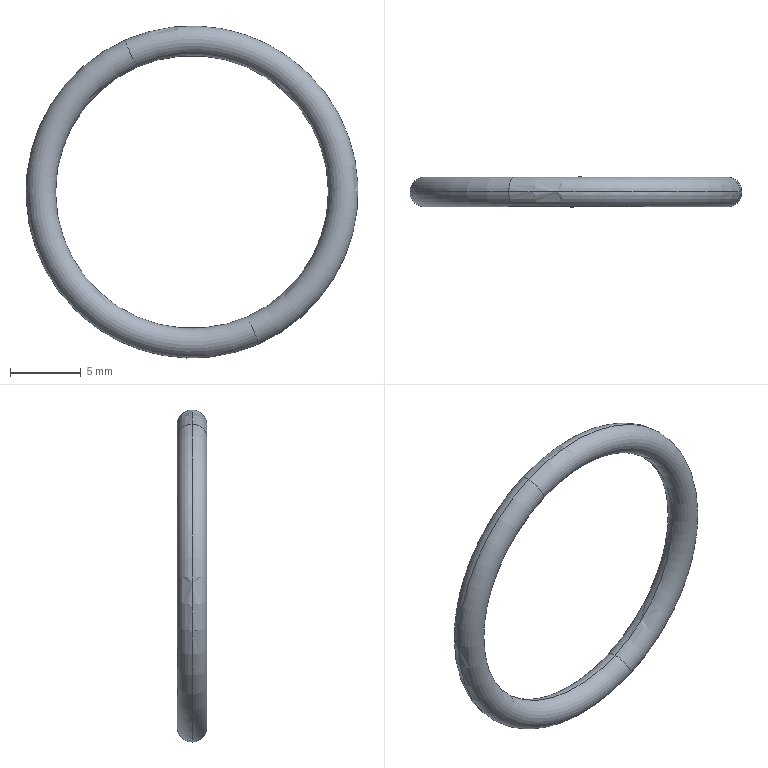Part | SolidWorks | features BaseBody 1 | 1 solid | 4 faces | box 23.5 x 2.1 x 23.5 mm | volume 232.859 mm3 | torus 4
STEP:
#1=CARTESIAN_POINT('',(224.737,118.05,10.742));
#2=VERTEX_POINT('',#1);
#3=CARTESIAN_POINT('',(225.589,118.05,8.822));
#4=VERTEX_POINT('',#3);
#5=CARTESIAN_POINT('',(225.163,118.05,9.782));
#6=DIRECTION('',(0.9142,0.,0.4053));
#7=DIRECTION('',(0.4053,0.,-0.9142));
#8=AXIS2_PLACEMENT_3D('',#5,#6,#7);
#9=CIRCLE('',#8,1.05);
#10=EDGE_CURVE('',#2,#4,#9,.T.);
#11=ORIENTED_EDGE('',*,*,#10,.F.);
#12=CARTESIAN_POINT('',(234.263,118.05,-10.742));
#13=VERTEX_POINT('',#12);
#14=CARTESIAN_POINT('',(229.5,118.05,0.));
#15=DIRECTION('',(0.,-1.,0.));
#16=DIRECTION('',(0.,0.,-1.));
#17=AXIS2_PLACEMENT_3D('',#14,#15,#16);
#18=CIRCLE('',#17,11.75);
#19=EDGE_CURVE('',#2,#13,#18,.T.);
#20=ORIENTED_EDGE('',*,*,#19,.T.);
#21=CARTESIAN_POINT('',(233.411,118.05,-8.822));
#22=VERTEX_POINT('',#21);
#23=CARTESIAN_POINT('',(233.837,118.05,-9.782));
#24=DIRECTION('',(-0.9142,0.,-0.4053));
#25=DIRECTION('',(-0.4053,0.,0.9142));
#26=AXIS2_PLACEMENT_3D('',#23,#24,#25);
#27=CIRCLE('',#26,1.05);
#28=EDGE_CURVE('',#13,#22,#27,.T.);
#29=ORIENTED_EDGE('',*,*,#28,.T.);
#30=CARTESIAN_POINT('',(229.5,118.05,0.));
#31=DIRECTION('',(0.,-1.,0.));
#32=DIRECTION('',(0.,0.,-1.));
#33=AXIS2_PLACEMENT_3D('',#30,#31,#32);
#34=CIRCLE('',#33,9.65);
#35=EDGE_CURVE('',#4,#22,#34,.T.);
#36=ORIENTED_EDGE('',*,*,#35,.F.);
#37=EDGE_LOOP('',(#11,#20,#29,#36));
#38=FACE_OUTER_BOUND('',#37,.T.);
#39=CARTESIAN_POINT('',(229.5,118.05,0.));
#40=DIRECTION('',(0.,-1.,0.));
#41=DIRECTION('',(0.4053,0.,-0.9142));
#42=AXIS2_PLACEMENT_3D('',#39,#40,#41);
#43=TOROIDAL_SURFACE('',#42,10.7,1.05);
#44=ADVANCED_FACE('',(#38),#43,.T.);
#45=ORIENTED_EDGE('',*,*,#28,.F.);
#46=CARTESIAN_POINT('',(229.5,118.05,0.));
#47=DIRECTION('',(0.,-1.,0.));
#48=DIRECTION('',(0.,0.,-1.));
#49=AXIS2_PLACEMENT_3D('',#46,#47,#48);
#50=CIRCLE('',#49,11.75);
#51=EDGE_CURVE('',#13,#2,#50,.T.);
#52=ORIENTED_EDGE('',*,*,#51,.T.);
#53=ORIENTED_EDGE('',*,*,#10,.T.);
#54=CARTESIAN_POINT('',(229.5,118.05,0.));
#55=DIRECTION('',(0.,-1.,0.));
#56=DIRECTION('',(0.,0.,-1.));
#57=AXIS2_PLACEMENT_3D('',#54,#55,#56);
#58=CIRCLE('',#57,9.65);
#59=EDGE_CURVE('',#22,#4,#58,.T.);
#60=ORIENTED_EDGE('',*,*,#59,.F.);
#61=EDGE_LOOP('',(#45,#52,#53,#60));
#62=FACE_OUTER_BOUND('',#61,.T.);
#63=CARTESIAN_POINT('',(229.5,118.05,0.));
#64=DIRECTION('',(0.,-1.,0.));
#65=DIRECTION('',(0.4053,0.,-0.9142));
#66=AXIS2_PLACEMENT_3D('',#63,#64,#65);
#67=TOROIDAL_SURFACE('',#66,10.7,1.05);
#68=ADVANCED_FACE('',(#62),#67,.T.);
#69=ORIENTED_EDGE('',*,*,#51,.F.);
#70=CARTESIAN_POINT('',(233.837,118.05,-9.782));
#71=DIRECTION('',(-0.9142,0.,-0.4053));
#72=DIRECTION('',(-0.4053,0.,0.9142));
#73=AXIS2_PLACEMENT_3D('',#70,#71,#72);
#74=CIRCLE('',#73,1.05);
#75=EDGE_CURVE('',#22,#13,#74,.T.);
#76=ORIENTED_EDGE('',*,*,#75,.F.);
#77=ORIENTED_EDGE('',*,*,#59,.T.);
#78=CARTESIAN_POINT('',(225.163,118.05,9.782));
#79=DIRECTION('',(0.9142,0.,0.4053));
#80=DIRECTION('',(0.4053,0.,-0.9142));
#81=AXIS2_PLACEMENT_3D('',#78,#79,#80);
#82=CIRCLE('',#81,1.05);
#83=EDGE_CURVE('',#4,#2,#82,.T.);
#84=ORIENTED_EDGE('',*,*,#83,.T.);
#85=EDGE_LOOP('',(#69,#76,#77,#84));
#86=FACE_OUTER_BOUND('',#85,.T.);
#87=CARTESIAN_POINT('',(229.5,118.05,0.));
#88=DIRECTION('',(0.,-1.,0.));
#89=DIRECTION('',(0.4053,0.,-0.9142));
#90=AXIS2_PLACEMENT_3D('',#87,#88,#89);
#91=TOROIDAL_SURFACE('',#90,10.7,1.05);
#92=ADVANCED_FACE('',(#86),#91,.T.);
#93=ORIENTED_EDGE('',*,*,#19,.F.);
#94=ORIENTED_EDGE('',*,*,#83,.F.);
#95=ORIENTED_EDGE('',*,*,#35,.T.);
#96=ORIENTED_EDGE('',*,*,#75,.T.);
#97=EDGE_LOOP('',(#93,#94,#95,#96));
#98=FACE_OUTER_BOUND('',#97,.T.);
#99=CARTESIAN_POINT('',(229.5,118.05,0.));
#100=DIRECTION('',(0.,-1.,0.));
#101=DIRECTION('',(0.4053,0.,-0.9142));
#102=AXIS2_PLACEMENT_3D('',#99,#100,#101);
#103=TOROIDAL_SURFACE('',#102,10.7,1.05);
#104=ADVANCED_FACE('',(#98),#103,.T.);
#105=CLOSED_SHELL('',(#44,#68,#92,#104));
#106=MANIFOLD_SOLID_BREP('',#105);
#107=CARTESIAN_POINT('',(0.,0.,0.));
#108=DIRECTION('',(0.,0.,1.));
#109=DIRECTION('',(1.,0.,0.));
#110=AXIS2_PLACEMENT_3D('',#107,#108,#109);
#111=(LENGTH_UNIT()NAMED_UNIT(*)SI_UNIT(.MILLI.,.METRE.));
#112=UNCERTAINTY_MEASURE_WITH_UNIT(LENGTH_MEASURE(0.00001),#111,'','');
#113=(NAMED_UNIT(*)PLANE_ANGLE_UNIT()SI_UNIT($,.RADIAN.));
#114=(NAMED_UNIT(*)SI_UNIT($,.STERADIAN.)SOLID_ANGLE_UNIT());
#115=(GEOMETRIC_REPRESENTATION_CONTEXT(3)GLOBAL_UNCERTAINTY_ASSIGNED_CONTEXT((#112))GLOBAL_UNIT_ASSIGNED_CONTEXT((#111,#113,#114))REPRESENTATION_CONTEXT('',''));
#116=ADVANCED_BREP_SHAPE_REPRESENTATION('',(#106,#110),#115);